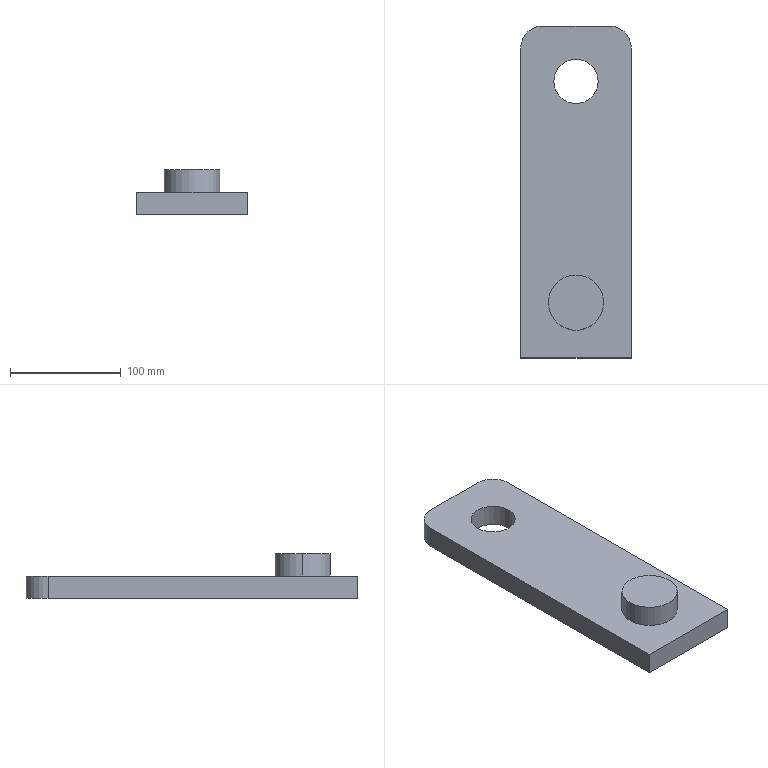Part | SolidWorks | features Extrusion 1, Fillet 1, ICE 1 | 1 solid | 13 faces | box 100 x 300 x 40 mm | volume 610704 mm3 | plane 7 | cylinder 6 | commonest cylinder face diameters 40 x4 50 x2
STEP:
#1=CARTESIAN_POINT('',(20.,200.,-20.));
#2=VERTEX_POINT('',#1);
#3=CARTESIAN_POINT('',(-20.,200.,-20.));
#4=VERTEX_POINT('',#3);
#5=CARTESIAN_POINT('',(0.,200.,-20.));
#6=DIRECTION('',(0.,0.,-1.));
#7=DIRECTION('',(-1.,0.,0.));
#8=AXIS2_PLACEMENT_3D('',#5,#6,#7);
#9=CIRCLE('',#8,20.);
#10=EDGE_CURVE('',#2,#4,#9,.T.);
#11=ORIENTED_EDGE('',*,*,#10,.T.);
#12=CARTESIAN_POINT('',(-20.,200.,0.));
#13=VERTEX_POINT('',#12);
#14=CARTESIAN_POINT('',(-20.,200.,-20.));
#15=DIRECTION('',(0.,0.,1.));
#16=VECTOR('',#15,1000.);
#17=LINE('',#14,#16);
#18=EDGE_CURVE('',#4,#13,#17,.T.);
#19=ORIENTED_EDGE('',*,*,#18,.T.);
#20=CARTESIAN_POINT('',(20.,200.,0.));
#21=VERTEX_POINT('',#20);
#22=CARTESIAN_POINT('',(0.,200.,0.));
#23=DIRECTION('',(0.,0.,-1.));
#24=DIRECTION('',(-1.,0.,0.));
#25=AXIS2_PLACEMENT_3D('',#22,#23,#24);
#26=CIRCLE('',#25,20.);
#27=EDGE_CURVE('',#21,#13,#26,.T.);
#28=ORIENTED_EDGE('',*,*,#27,.F.);
#29=CARTESIAN_POINT('',(20.,200.,-20.));
#30=DIRECTION('',(0.,0.,1.));
#31=VECTOR('',#30,1000.);
#32=LINE('',#29,#31);
#33=EDGE_CURVE('',#2,#21,#32,.T.);
#34=ORIENTED_EDGE('',*,*,#33,.F.);
#35=EDGE_LOOP('',(#11,#19,#28,#34));
#36=FACE_OUTER_BOUND('',#35,.T.);
#37=CARTESIAN_POINT('',(0.,200.,-20.));
#38=DIRECTION('',(0.,0.,1.));
#39=DIRECTION('',(1.,0.,0.));
#40=AXIS2_PLACEMENT_3D('',#37,#38,#39);
#41=CYLINDRICAL_SURFACE('',#40,20.);
#42=ADVANCED_FACE('',(#36),#41,.F.);
#43=CARTESIAN_POINT('',(25.,0.,20.));
#44=VERTEX_POINT('',#43);
#45=CARTESIAN_POINT('',(-25.,0.,20.));
#46=VERTEX_POINT('',#45);
#47=CARTESIAN_POINT('',(0.,0.,20.));
#48=DIRECTION('',(0.,0.,1.));
#49=DIRECTION('',(1.,0.,0.));
#50=AXIS2_PLACEMENT_3D('',#47,#48,#49);
#51=CIRCLE('',#50,25.);
#52=EDGE_CURVE('',#44,#46,#51,.T.);
#53=ORIENTED_EDGE('',*,*,#52,.F.);
#54=CARTESIAN_POINT('',(25.,0.,0.));
#55=VERTEX_POINT('',#54);
#56=CARTESIAN_POINT('',(25.,0.,20.));
#57=DIRECTION('',(0.,0.,-1.));
#58=VECTOR('',#57,1000.);
#59=LINE('',#56,#58);
#60=EDGE_CURVE('',#44,#55,#59,.T.);
#61=ORIENTED_EDGE('',*,*,#60,.T.);
#62=CARTESIAN_POINT('',(-25.,0.,0.));
#63=VERTEX_POINT('',#62);
#64=CARTESIAN_POINT('',(0.,0.,0.));
#65=DIRECTION('',(0.,0.,1.));
#66=DIRECTION('',(1.,0.,0.));
#67=AXIS2_PLACEMENT_3D('',#64,#65,#66);
#68=CIRCLE('',#67,25.);
#69=EDGE_CURVE('',#55,#63,#68,.T.);
#70=ORIENTED_EDGE('',*,*,#69,.T.);
#71=CARTESIAN_POINT('',(-25.,0.,20.));
#72=DIRECTION('',(0.,0.,-1.));
#73=VECTOR('',#72,1000.);
#74=LINE('',#71,#73);
#75=EDGE_CURVE('',#46,#63,#74,.T.);
#76=ORIENTED_EDGE('',*,*,#75,.F.);
#77=EDGE_LOOP('',(#53,#61,#70,#76));
#78=FACE_OUTER_BOUND('',#77,.T.);
#79=CARTESIAN_POINT('',(0.,0.,20.));
#80=DIRECTION('',(0.,0.,-1.));
#81=DIRECTION('',(-1.,0.,0.));
#82=AXIS2_PLACEMENT_3D('',#79,#80,#81);
#83=CYLINDRICAL_SURFACE('',#82,25.);
#84=ADVANCED_FACE('',(#78),#83,.T.);
#85=ORIENTED_EDGE('',*,*,#60,.F.);
#86=CARTESIAN_POINT('',(0.,0.,20.));
#87=DIRECTION('',(0.,0.,1.));
#88=DIRECTION('',(1.,0.,0.));
#89=AXIS2_PLACEMENT_3D('',#86,#87,#88);
#90=CIRCLE('',#89,25.);
#91=EDGE_CURVE('',#46,#44,#90,.T.);
#92=ORIENTED_EDGE('',*,*,#91,.F.);
#93=ORIENTED_EDGE('',*,*,#75,.T.);
#94=CARTESIAN_POINT('',(0.,0.,0.));
#95=DIRECTION('',(0.,0.,1.));
#96=DIRECTION('',(1.,0.,0.));
#97=AXIS2_PLACEMENT_3D('',#94,#95,#96);
#98=CIRCLE('',#97,25.);
#99=EDGE_CURVE('',#63,#55,#98,.T.);
#100=ORIENTED_EDGE('',*,*,#99,.T.);
#101=EDGE_LOOP('',(#85,#92,#93,#100));
#102=FACE_OUTER_BOUND('',#101,.T.);
#103=CARTESIAN_POINT('',(0.,0.,20.));
#104=DIRECTION('',(0.,0.,-1.));
#105=DIRECTION('',(-1.,0.,0.));
#106=AXIS2_PLACEMENT_3D('',#103,#104,#105);
#107=CYLINDRICAL_SURFACE('',#106,25.);
#108=ADVANCED_FACE('',(#102),#107,.T.);
#109=ORIENTED_EDGE('',*,*,#91,.T.);
#110=ORIENTED_EDGE('',*,*,#52,.T.);
#111=EDGE_LOOP('',(#109,#110));
#112=FACE_OUTER_BOUND('',#111,.T.);
#113=CARTESIAN_POINT('',(0.,0.,20.));
#114=DIRECTION('',(0.,0.,1.));
#115=DIRECTION('',(1.,0.,0.));
#116=AXIS2_PLACEMENT_3D('',#113,#114,#115);
#117=PLANE('',#116);
#118=ADVANCED_FACE('',(#112),#117,.T.);
#119=CARTESIAN_POINT('',(-50.,-50.,-20.));
#120=VERTEX_POINT('',#119);
#121=CARTESIAN_POINT('',(-50.,230.,-20.));
#122=VERTEX_POINT('',#121);
#123=CARTESIAN_POINT('',(-50.,250.,-20.));
#124=DIRECTION('',(0.,1.,0.));
#125=VECTOR('',#124,1000.);
#126=LINE('',#123,#125);
#127=EDGE_CURVE('',#120,#122,#126,.T.);
#128=ORIENTED_EDGE('',*,*,#127,.T.);
#129=CARTESIAN_POINT('',(-30.,250.,-20.));
#130=VERTEX_POINT('',#129);
#131=CARTESIAN_POINT('',(-30.,230.,-20.));
#132=DIRECTION('',(0.,0.,-1.));
#133=DIRECTION('',(-1.,0.,0.));
#134=AXIS2_PLACEMENT_3D('',#131,#132,#133);
#135=CIRCLE('',#134,20.);
#136=EDGE_CURVE('',#122,#130,#135,.T.);
#137=ORIENTED_EDGE('',*,*,#136,.T.);
#138=CARTESIAN_POINT('',(30.,250.,-20.));
#139=VERTEX_POINT('',#138);
#140=CARTESIAN_POINT('',(50.,250.,-20.));
#141=DIRECTION('',(1.,0.,0.));
#142=VECTOR('',#141,1000.);
#143=LINE('',#140,#142);
#144=EDGE_CURVE('',#130,#139,#143,.T.);
#145=ORIENTED_EDGE('',*,*,#144,.T.);
#146=CARTESIAN_POINT('',(50.,230.,-20.));
#147=VERTEX_POINT('',#146);
#148=CARTESIAN_POINT('',(30.,230.,-20.));
#149=DIRECTION('',(0.,0.,-1.));
#150=DIRECTION('',(-1.,0.,0.));
#151=AXIS2_PLACEMENT_3D('',#148,#149,#150);
#152=CIRCLE('',#151,20.);
#153=EDGE_CURVE('',#139,#147,#152,.T.);
#154=ORIENTED_EDGE('',*,*,#153,.T.);
#155=CARTESIAN_POINT('',(50.,-50.,-20.));
#156=VERTEX_POINT('',#155);
#157=CARTESIAN_POINT('',(50.,250.,-20.));
#158=DIRECTION('',(0.,-1.,0.));
#159=VECTOR('',#158,1000.);
#160=LINE('',#157,#159);
#161=EDGE_CURVE('',#147,#156,#160,.T.);
#162=ORIENTED_EDGE('',*,*,#161,.T.);
#163=CARTESIAN_POINT('',(50.,-50.,-20.));
#164=DIRECTION('',(-1.,0.,0.));
#165=VECTOR('',#164,1000.);
#166=LINE('',#163,#165);
#167=EDGE_CURVE('',#156,#120,#166,.T.);
#168=ORIENTED_EDGE('',*,*,#167,.T.);
#169=EDGE_LOOP('',(#128,#137,#145,#154,#162,#168));
#170=FACE_OUTER_BOUND('',#169,.T.);
#171=ORIENTED_EDGE('',*,*,#10,.F.);
#172=CARTESIAN_POINT('',(0.,200.,-20.));
#173=DIRECTION('',(0.,0.,-1.));
#174=DIRECTION('',(-1.,0.,0.));
#175=AXIS2_PLACEMENT_3D('',#172,#173,#174);
#176=CIRCLE('',#175,20.);
#177=EDGE_CURVE('',#4,#2,#176,.T.);
#178=ORIENTED_EDGE('',*,*,#177,.F.);
#179=EDGE_LOOP('',(#171,#178));
#180=FACE_BOUND('',#179,.T.);
#181=CARTESIAN_POINT('',(0.,0.,-20.));
#182=DIRECTION('',(0.,0.,-1.));
#183=DIRECTION('',(-1.,0.,0.));
#184=AXIS2_PLACEMENT_3D('',#181,#182,#183);
#185=PLANE('',#184);
#186=ADVANCED_FACE('',(#170,#180),#185,.T.);
#187=ORIENTED_EDGE('',*,*,#99,.F.);
#188=ORIENTED_EDGE('',*,*,#69,.F.);
#189=EDGE_LOOP('',(#187,#188));
#190=FACE_BOUND('',#189,.T.);
#191=CARTESIAN_POINT('',(-30.,250.,0.));
#192=VERTEX_POINT('',#191);
#193=CARTESIAN_POINT('',(30.,250.,0.));
#194=VERTEX_POINT('',#193);
#195=CARTESIAN_POINT('',(50.,250.,0.));
#196=DIRECTION('',(1.,0.,0.));
#197=VECTOR('',#196,1000.);
#198=LINE('',#195,#197);
#199=EDGE_CURVE('',#192,#194,#198,.T.);
#200=ORIENTED_EDGE('',*,*,#199,.F.);
#201=CARTESIAN_POINT('',(-50.,230.,0.));
#202=VERTEX_POINT('',#201);
#203=CARTESIAN_POINT('',(-30.,230.,0.));
#204=DIRECTION('',(0.,0.,1.));
#205=DIRECTION('',(-1.,0.,0.));
#206=AXIS2_PLACEMENT_3D('',#203,#204,#205);
#207=CIRCLE('',#206,20.);
#208=EDGE_CURVE('',#192,#202,#207,.T.);
#209=ORIENTED_EDGE('',*,*,#208,.T.);
#210=CARTESIAN_POINT('',(-50.,-50.,0.));
#211=VERTEX_POINT('',#210);
#212=CARTESIAN_POINT('',(-50.,250.,0.));
#213=DIRECTION('',(0.,1.,0.));
#214=VECTOR('',#213,1000.);
#215=LINE('',#212,#214);
#216=EDGE_CURVE('',#211,#202,#215,.T.);
#217=ORIENTED_EDGE('',*,*,#216,.F.);
#218=CARTESIAN_POINT('',(50.,-50.,0.));
#219=VERTEX_POINT('',#218);
#220=CARTESIAN_POINT('',(50.,-50.,0.));
#221=DIRECTION('',(-1.,0.,0.));
#222=VECTOR('',#221,1000.);
#223=LINE('',#220,#222);
#224=EDGE_CURVE('',#219,#211,#223,.T.);
#225=ORIENTED_EDGE('',*,*,#224,.F.);
#226=CARTESIAN_POINT('',(50.,230.,0.));
#227=VERTEX_POINT('',#226);
#228=CARTESIAN_POINT('',(50.,250.,0.));
#229=DIRECTION('',(0.,-1.,0.));
#230=VECTOR('',#229,1000.);
#231=LINE('',#228,#230);
#232=EDGE_CURVE('',#227,#219,#231,.T.);
#233=ORIENTED_EDGE('',*,*,#232,.F.);
#234=CARTESIAN_POINT('',(30.,230.,0.));
#235=DIRECTION('',(0.,0.,1.));
#236=DIRECTION('',(-1.,0.,0.));
#237=AXIS2_PLACEMENT_3D('',#234,#235,#236);
#238=CIRCLE('',#237,20.);
#239=EDGE_CURVE('',#227,#194,#238,.T.);
#240=ORIENTED_EDGE('',*,*,#239,.T.);
#241=EDGE_LOOP('',(#200,#209,#217,#225,#233,#240));
#242=FACE_OUTER_BOUND('',#241,.T.);
#243=ORIENTED_EDGE('',*,*,#27,.T.);
#244=CARTESIAN_POINT('',(0.,200.,0.));
#245=DIRECTION('',(0.,0.,-1.));
#246=DIRECTION('',(-1.,0.,0.));
#247=AXIS2_PLACEMENT_3D('',#244,#245,#246);
#248=CIRCLE('',#247,20.);
#249=EDGE_CURVE('',#13,#21,#248,.T.);
#250=ORIENTED_EDGE('',*,*,#249,.T.);
#251=EDGE_LOOP('',(#243,#250));
#252=FACE_BOUND('',#251,.T.);
#253=CARTESIAN_POINT('',(0.,0.,0.));
#254=DIRECTION('',(0.,0.,-1.));
#255=DIRECTION('',(-1.,0.,0.));
#256=AXIS2_PLACEMENT_3D('',#253,#254,#255);
#257=PLANE('',#256);
#258=ADVANCED_FACE('',(#190,#242,#252),#257,.F.);
#259=ORIENTED_EDGE('',*,*,#216,.T.);
#260=CARTESIAN_POINT('',(-50.,230.,-20.));
#261=DIRECTION('',(0.,0.,-1.));
#262=VECTOR('',#261,1000.);
#263=LINE('',#260,#262);
#264=EDGE_CURVE('',#202,#122,#263,.T.);
#265=ORIENTED_EDGE('',*,*,#264,.T.);
#266=ORIENTED_EDGE('',*,*,#127,.F.);
#267=CARTESIAN_POINT('',(-50.,-50.,-20.));
#268=DIRECTION('',(0.,0.,1.));
#269=VECTOR('',#268,1000.);
#270=LINE('',#267,#269);
#271=EDGE_CURVE('',#120,#211,#270,.T.);
#272=ORIENTED_EDGE('',*,*,#271,.T.);
#273=EDGE_LOOP('',(#259,#265,#266,#272));
#274=FACE_OUTER_BOUND('',#273,.T.);
#275=CARTESIAN_POINT('',(-50.,250.,-20.));
#276=DIRECTION('',(1.,0.,0.));
#277=DIRECTION('',(0.,1.,0.));
#278=AXIS2_PLACEMENT_3D('',#275,#276,#277);
#279=PLANE('',#278);
#280=ADVANCED_FACE('',(#274),#279,.F.);
#281=ORIENTED_EDGE('',*,*,#144,.F.);
#282=CARTESIAN_POINT('',(-30.,250.,-20.));
#283=DIRECTION('',(0.,0.,1.));
#284=VECTOR('',#283,1000.);
#285=LINE('',#282,#284);
#286=EDGE_CURVE('',#130,#192,#285,.T.);
#287=ORIENTED_EDGE('',*,*,#286,.T.);
#288=ORIENTED_EDGE('',*,*,#199,.T.);
#289=CARTESIAN_POINT('',(30.,250.,-20.));
#290=DIRECTION('',(0.,0.,-1.));
#291=VECTOR('',#290,1000.);
#292=LINE('',#289,#291);
#293=EDGE_CURVE('',#194,#139,#292,.T.);
#294=ORIENTED_EDGE('',*,*,#293,.T.);
#295=EDGE_LOOP('',(#281,#287,#288,#294));
#296=FACE_OUTER_BOUND('',#295,.T.);
#297=CARTESIAN_POINT('',(50.,250.,-20.));
#298=DIRECTION('',(0.,-1.,0.));
#299=DIRECTION('',(0.,0.,-1.));
#300=AXIS2_PLACEMENT_3D('',#297,#298,#299);
#301=PLANE('',#300);
#302=ADVANCED_FACE('',(#296),#301,.F.);
#303=ORIENTED_EDGE('',*,*,#161,.F.);
#304=CARTESIAN_POINT('',(50.,230.,-20.));
#305=DIRECTION('',(0.,0.,1.));
#306=VECTOR('',#305,1000.);
#307=LINE('',#304,#306);
#308=EDGE_CURVE('',#147,#227,#307,.T.);
#309=ORIENTED_EDGE('',*,*,#308,.T.);
#310=ORIENTED_EDGE('',*,*,#232,.T.);
#311=CARTESIAN_POINT('',(50.,-50.,-20.));
#312=DIRECTION('',(0.,0.,1.));
#313=VECTOR('',#312,1000.);
#314=LINE('',#311,#313);
#315=EDGE_CURVE('',#156,#219,#314,.T.);
#316=ORIENTED_EDGE('',*,*,#315,.F.);
#317=EDGE_LOOP('',(#303,#309,#310,#316));
#318=FACE_OUTER_BOUND('',#317,.T.);
#319=CARTESIAN_POINT('',(50.,250.,-20.));
#320=DIRECTION('',(-1.,0.,0.));
#321=DIRECTION('',(0.,-1.,0.));
#322=AXIS2_PLACEMENT_3D('',#319,#320,#321);
#323=PLANE('',#322);
#324=ADVANCED_FACE('',(#318),#323,.F.);
#325=ORIENTED_EDGE('',*,*,#224,.T.);
#326=ORIENTED_EDGE('',*,*,#271,.F.);
#327=ORIENTED_EDGE('',*,*,#167,.F.);
#328=ORIENTED_EDGE('',*,*,#315,.T.);
#329=EDGE_LOOP('',(#325,#326,#327,#328));
#330=FACE_OUTER_BOUND('',#329,.T.);
#331=CARTESIAN_POINT('',(50.,-50.,-20.));
#332=DIRECTION('',(0.,1.,0.));
#333=DIRECTION('',(0.,0.,1.));
#334=AXIS2_PLACEMENT_3D('',#331,#332,#333);
#335=PLANE('',#334);
#336=ADVANCED_FACE('',(#330),#335,.F.);
#337=ORIENTED_EDGE('',*,*,#18,.F.);
#338=ORIENTED_EDGE('',*,*,#177,.T.);
#339=ORIENTED_EDGE('',*,*,#33,.T.);
#340=ORIENTED_EDGE('',*,*,#249,.F.);
#341=EDGE_LOOP('',(#337,#338,#339,#340));
#342=FACE_OUTER_BOUND('',#341,.T.);
#343=CARTESIAN_POINT('',(0.,200.,-20.));
#344=DIRECTION('',(0.,0.,1.));
#345=DIRECTION('',(1.,0.,0.));
#346=AXIS2_PLACEMENT_3D('',#343,#344,#345);
#347=CYLINDRICAL_SURFACE('',#346,20.);
#348=ADVANCED_FACE('',(#342),#347,.F.);
#349=ORIENTED_EDGE('',*,*,#136,.F.);
#350=ORIENTED_EDGE('',*,*,#264,.F.);
#351=ORIENTED_EDGE('',*,*,#208,.F.);
#352=ORIENTED_EDGE('',*,*,#286,.F.);
#353=EDGE_LOOP('',(#349,#350,#351,#352));
#354=FACE_OUTER_BOUND('',#353,.T.);
#355=CARTESIAN_POINT('',(-30.,230.,-20.));
#356=DIRECTION('',(0.,0.,1.));
#357=DIRECTION('',(1.,0.,0.));
#358=AXIS2_PLACEMENT_3D('',#355,#356,#357);
#359=CYLINDRICAL_SURFACE('',#358,20.);
#360=ADVANCED_FACE('',(#354),#359,.T.);
#361=ORIENTED_EDGE('',*,*,#153,.F.);
#362=ORIENTED_EDGE('',*,*,#293,.F.);
#363=ORIENTED_EDGE('',*,*,#239,.F.);
#364=ORIENTED_EDGE('',*,*,#308,.F.);
#365=EDGE_LOOP('',(#361,#362,#363,#364));
#366=FACE_OUTER_BOUND('',#365,.T.);
#367=CARTESIAN_POINT('',(30.,230.,-20.));
#368=DIRECTION('',(0.,0.,1.));
#369=DIRECTION('',(1.,0.,0.));
#370=AXIS2_PLACEMENT_3D('',#367,#368,#369);
#371=CYLINDRICAL_SURFACE('',#370,20.);
#372=ADVANCED_FACE('',(#366),#371,.T.);
#373=CLOSED_SHELL('',(#42,#84,#108,#118,#186,#258,#280,#302,#324,#336,#348,#360,#372));
#374=MANIFOLD_SOLID_BREP('',#373);
#375=CARTESIAN_POINT('',(0.,0.,0.));
#376=DIRECTION('',(0.,0.,1.));
#377=DIRECTION('',(1.,0.,0.));
#378=AXIS2_PLACEMENT_3D('',#375,#376,#377);
#379=(LENGTH_UNIT()NAMED_UNIT(*)SI_UNIT(.MILLI.,.METRE.));
#380=UNCERTAINTY_MEASURE_WITH_UNIT(LENGTH_MEASURE(0.00001),#379,'','');
#381=(NAMED_UNIT(*)PLANE_ANGLE_UNIT()SI_UNIT($,.RADIAN.));
#382=(NAMED_UNIT(*)SI_UNIT($,.STERADIAN.)SOLID_ANGLE_UNIT());
#383=(GEOMETRIC_REPRESENTATION_CONTEXT(3)GLOBAL_UNCERTAINTY_ASSIGNED_CONTEXT((#380))GLOBAL_UNIT_ASSIGNED_CONTEXT((#379,#381,#382))REPRESENTATION_CONTEXT('',''));
#384=ADVANCED_BREP_SHAPE_REPRESENTATION('',(#374,#378),#383);